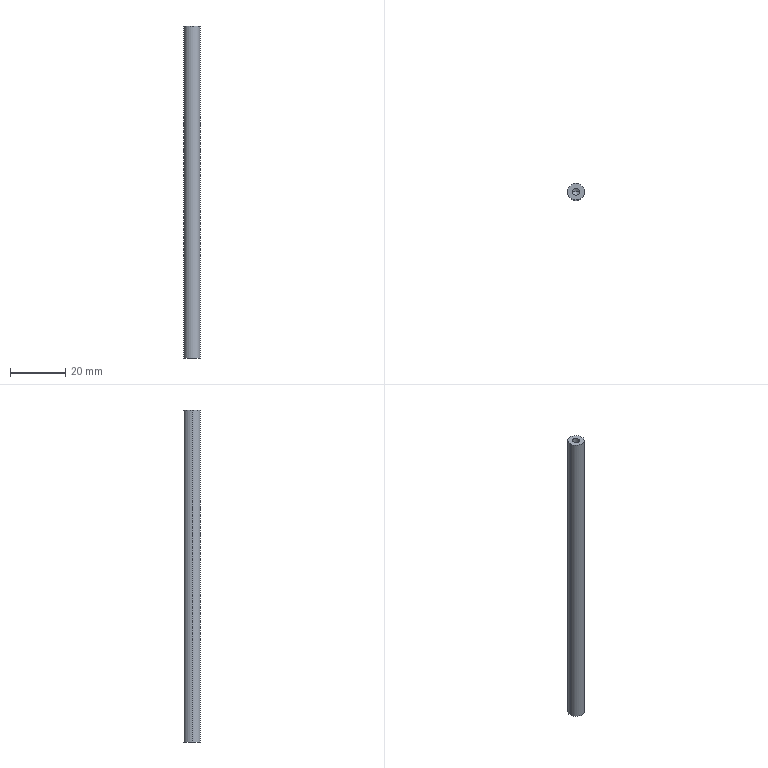Part | SolidWorks | features HoleWzd 2, Extrusion 1 | 1 solid | 12 faces | box 6 x 6 x 120 mm | volume 3307 mm3 | cylinder 6 | cone 4 | plane 2 | commonest cylinder face diameters 2.5 x4 6 x2
STEP:
#1=CARTESIAN_POINT('',(1.25,0.,8.5));
#2=VERTEX_POINT('',#1);
#3=CARTESIAN_POINT('',(-1.25,0.,8.5));
#4=VERTEX_POINT('',#3);
#5=CARTESIAN_POINT('',(0.,0.,8.5));
#6=DIRECTION('',(0.,0.,-1.));
#7=DIRECTION('',(-1.,0.,0.));
#8=AXIS2_PLACEMENT_3D('',#5,#6,#7);
#9=CIRCLE('',#8,1.25);
#10=EDGE_CURVE('',#2,#4,#9,.T.);
#11=ORIENTED_EDGE('',*,*,#10,.F.);
#12=CARTESIAN_POINT('',(1.25,0.,0.));
#13=VERTEX_POINT('',#12);
#14=CARTESIAN_POINT('',(1.25,0.,0.));
#15=DIRECTION('',(0.,0.,-1.));
#16=VECTOR('',#15,1000.);
#17=LINE('',#14,#16);
#18=EDGE_CURVE('',#2,#13,#17,.T.);
#19=ORIENTED_EDGE('',*,*,#18,.T.);
#20=CARTESIAN_POINT('',(-1.25,0.,0.));
#21=VERTEX_POINT('',#20);
#22=CARTESIAN_POINT('',(0.,0.,0.));
#23=DIRECTION('',(0.,0.,-1.));
#24=DIRECTION('',(-1.,0.,0.));
#25=AXIS2_PLACEMENT_3D('',#22,#23,#24);
#26=CIRCLE('',#25,1.25);
#27=EDGE_CURVE('',#13,#21,#26,.T.);
#28=ORIENTED_EDGE('',*,*,#27,.T.);
#29=CARTESIAN_POINT('',(-1.25,0.,0.));
#30=DIRECTION('',(0.,0.,-1.));
#31=VECTOR('',#30,1000.);
#32=LINE('',#29,#31);
#33=EDGE_CURVE('',#4,#21,#32,.T.);
#34=ORIENTED_EDGE('',*,*,#33,.F.);
#35=EDGE_LOOP('',(#11,#19,#28,#34));
#36=FACE_OUTER_BOUND('',#35,.T.);
#37=CARTESIAN_POINT('',(0.,0.,0.));
#38=DIRECTION('',(0.,0.,-1.));
#39=DIRECTION('',(-1.,0.,0.));
#40=AXIS2_PLACEMENT_3D('',#37,#38,#39);
#41=CYLINDRICAL_SURFACE('',#40,1.25);
#42=ADVANCED_FACE('',(#36),#41,.F.);
#43=CARTESIAN_POINT('',(0.,0.,9.251));
#44=VERTEX_POINT('',#43);
#45=CARTESIAN_POINT('',(-1.25,0.,8.5));
#46=DIRECTION('',(-0.8572,0.,-0.515));
#47=VECTOR('',#46,1000.);
#48=LINE('',#45,#47);
#49=EDGE_CURVE('',#44,#4,#48,.T.);
#50=ORIENTED_EDGE('',*,*,#49,.F.);
#51=CARTESIAN_POINT('',(1.25,0.,8.5));
#52=DIRECTION('',(0.8572,0.,-0.515));
#53=VECTOR('',#52,1000.);
#54=LINE('',#51,#53);
#55=EDGE_CURVE('',#44,#2,#54,.T.);
#56=ORIENTED_EDGE('',*,*,#55,.T.);
#57=ORIENTED_EDGE('',*,*,#10,.T.);
#58=EDGE_LOOP('',(#50,#56,#57));
#59=FACE_OUTER_BOUND('',#58,.T.);
#60=CARTESIAN_POINT('',(0.,0.,8.5));
#61=DIRECTION('',(0.,0.,-1.));
#62=DIRECTION('',(-1.,0.,0.));
#63=AXIS2_PLACEMENT_3D('',#60,#61,#62);
#64=CONICAL_SURFACE('',#63,1.25,1.03);
#65=ADVANCED_FACE('',(#59),#64,.F.);
#66=CARTESIAN_POINT('',(-1.25,0.,111.5));
#67=VERTEX_POINT('',#66);
#68=CARTESIAN_POINT('',(1.25,0.,111.5));
#69=VERTEX_POINT('',#68);
#70=CARTESIAN_POINT('',(0.,0.,111.5));
#71=DIRECTION('',(0.,0.,1.));
#72=DIRECTION('',(1.,0.,0.));
#73=AXIS2_PLACEMENT_3D('',#70,#71,#72);
#74=CIRCLE('',#73,1.25);
#75=EDGE_CURVE('',#67,#69,#74,.T.);
#76=ORIENTED_EDGE('',*,*,#75,.F.);
#77=CARTESIAN_POINT('',(-1.25,0.,120.));
#78=VERTEX_POINT('',#77);
#79=CARTESIAN_POINT('',(-1.25,0.,120.));
#80=DIRECTION('',(0.,0.,1.));
#81=VECTOR('',#80,1000.);
#82=LINE('',#79,#81);
#83=EDGE_CURVE('',#67,#78,#82,.T.);
#84=ORIENTED_EDGE('',*,*,#83,.T.);
#85=CARTESIAN_POINT('',(1.25,0.,120.));
#86=VERTEX_POINT('',#85);
#87=CARTESIAN_POINT('',(0.,0.,120.));
#88=DIRECTION('',(0.,0.,1.));
#89=DIRECTION('',(1.,0.,0.));
#90=AXIS2_PLACEMENT_3D('',#87,#88,#89);
#91=CIRCLE('',#90,1.25);
#92=EDGE_CURVE('',#78,#86,#91,.T.);
#93=ORIENTED_EDGE('',*,*,#92,.T.);
#94=CARTESIAN_POINT('',(1.25,0.,120.));
#95=DIRECTION('',(0.,0.,1.));
#96=VECTOR('',#95,1000.);
#97=LINE('',#94,#96);
#98=EDGE_CURVE('',#69,#86,#97,.T.);
#99=ORIENTED_EDGE('',*,*,#98,.F.);
#100=EDGE_LOOP('',(#76,#84,#93,#99));
#101=FACE_OUTER_BOUND('',#100,.T.);
#102=CARTESIAN_POINT('',(0.,0.,120.));
#103=DIRECTION('',(0.,0.,1.));
#104=DIRECTION('',(1.,0.,0.));
#105=AXIS2_PLACEMENT_3D('',#102,#103,#104);
#106=CYLINDRICAL_SURFACE('',#105,1.25);
#107=ADVANCED_FACE('',(#101),#106,.F.);
#108=CARTESIAN_POINT('',(0.,0.,110.749));
#109=VERTEX_POINT('',#108);
#110=CARTESIAN_POINT('',(1.25,0.,111.5));
#111=DIRECTION('',(0.8572,0.,0.515));
#112=VECTOR('',#111,1000.);
#113=LINE('',#110,#112);
#114=EDGE_CURVE('',#109,#69,#113,.T.);
#115=ORIENTED_EDGE('',*,*,#114,.F.);
#116=CARTESIAN_POINT('',(-1.25,0.,111.5));
#117=DIRECTION('',(-0.8572,0.,0.515));
#118=VECTOR('',#117,1000.);
#119=LINE('',#116,#118);
#120=EDGE_CURVE('',#109,#67,#119,.T.);
#121=ORIENTED_EDGE('',*,*,#120,.T.);
#122=ORIENTED_EDGE('',*,*,#75,.T.);
#123=EDGE_LOOP('',(#115,#121,#122));
#124=FACE_OUTER_BOUND('',#123,.T.);
#125=CARTESIAN_POINT('',(0.,0.,111.5));
#126=DIRECTION('',(0.,0.,1.));
#127=DIRECTION('',(1.,0.,0.));
#128=AXIS2_PLACEMENT_3D('',#125,#126,#127);
#129=CONICAL_SURFACE('',#128,1.25,1.03);
#130=ADVANCED_FACE('',(#124),#129,.F.);
#131=CARTESIAN_POINT('',(3.,0.,120.));
#132=VERTEX_POINT('',#131);
#133=CARTESIAN_POINT('',(-3.,0.,120.));
#134=VERTEX_POINT('',#133);
#135=CARTESIAN_POINT('',(0.,0.,120.));
#136=DIRECTION('',(0.,0.,1.));
#137=DIRECTION('',(1.,0.,0.));
#138=AXIS2_PLACEMENT_3D('',#135,#136,#137);
#139=CIRCLE('',#138,3.);
#140=EDGE_CURVE('',#132,#134,#139,.T.);
#141=ORIENTED_EDGE('',*,*,#140,.F.);
#142=CARTESIAN_POINT('',(3.,0.,0.));
#143=VERTEX_POINT('',#142);
#144=CARTESIAN_POINT('',(3.,0.,120.));
#145=DIRECTION('',(0.,0.,-1.));
#146=VECTOR('',#145,1000.);
#147=LINE('',#144,#146);
#148=EDGE_CURVE('',#132,#143,#147,.T.);
#149=ORIENTED_EDGE('',*,*,#148,.T.);
#150=CARTESIAN_POINT('',(-3.,0.,0.));
#151=VERTEX_POINT('',#150);
#152=CARTESIAN_POINT('',(0.,0.,0.));
#153=DIRECTION('',(0.,0.,1.));
#154=DIRECTION('',(1.,0.,0.));
#155=AXIS2_PLACEMENT_3D('',#152,#153,#154);
#156=CIRCLE('',#155,3.);
#157=EDGE_CURVE('',#143,#151,#156,.T.);
#158=ORIENTED_EDGE('',*,*,#157,.T.);
#159=CARTESIAN_POINT('',(-3.,0.,120.));
#160=DIRECTION('',(0.,0.,-1.));
#161=VECTOR('',#160,1000.);
#162=LINE('',#159,#161);
#163=EDGE_CURVE('',#134,#151,#162,.T.);
#164=ORIENTED_EDGE('',*,*,#163,.F.);
#165=EDGE_LOOP('',(#141,#149,#158,#164));
#166=FACE_OUTER_BOUND('',#165,.T.);
#167=CARTESIAN_POINT('',(0.,0.,120.));
#168=DIRECTION('',(0.,0.,-1.));
#169=DIRECTION('',(-1.,0.,0.));
#170=AXIS2_PLACEMENT_3D('',#167,#168,#169);
#171=CYLINDRICAL_SURFACE('',#170,3.);
#172=ADVANCED_FACE('',(#166),#171,.T.);
#173=ORIENTED_EDGE('',*,*,#148,.F.);
#174=CARTESIAN_POINT('',(0.,0.,120.));
#175=DIRECTION('',(0.,0.,1.));
#176=DIRECTION('',(1.,0.,0.));
#177=AXIS2_PLACEMENT_3D('',#174,#175,#176);
#178=CIRCLE('',#177,3.);
#179=EDGE_CURVE('',#134,#132,#178,.T.);
#180=ORIENTED_EDGE('',*,*,#179,.F.);
#181=ORIENTED_EDGE('',*,*,#163,.T.);
#182=CARTESIAN_POINT('',(0.,0.,0.));
#183=DIRECTION('',(0.,0.,1.));
#184=DIRECTION('',(1.,0.,0.));
#185=AXIS2_PLACEMENT_3D('',#182,#183,#184);
#186=CIRCLE('',#185,3.);
#187=EDGE_CURVE('',#151,#143,#186,.T.);
#188=ORIENTED_EDGE('',*,*,#187,.T.);
#189=EDGE_LOOP('',(#173,#180,#181,#188));
#190=FACE_OUTER_BOUND('',#189,.T.);
#191=CARTESIAN_POINT('',(0.,0.,120.));
#192=DIRECTION('',(0.,0.,-1.));
#193=DIRECTION('',(-1.,0.,0.));
#194=AXIS2_PLACEMENT_3D('',#191,#192,#193);
#195=CYLINDRICAL_SURFACE('',#194,3.);
#196=ADVANCED_FACE('',(#190),#195,.T.);
#197=CARTESIAN_POINT('',(0.,0.,120.));
#198=DIRECTION('',(0.,0.,1.));
#199=DIRECTION('',(1.,0.,0.));
#200=AXIS2_PLACEMENT_3D('',#197,#198,#199);
#201=CIRCLE('',#200,1.25);
#202=EDGE_CURVE('',#86,#78,#201,.T.);
#203=ORIENTED_EDGE('',*,*,#202,.F.);
#204=ORIENTED_EDGE('',*,*,#92,.F.);
#205=EDGE_LOOP('',(#203,#204));
#206=FACE_BOUND('',#205,.T.);
#207=ORIENTED_EDGE('',*,*,#179,.T.);
#208=ORIENTED_EDGE('',*,*,#140,.T.);
#209=EDGE_LOOP('',(#207,#208));
#210=FACE_OUTER_BOUND('',#209,.T.);
#211=CARTESIAN_POINT('',(0.,0.,120.));
#212=DIRECTION('',(0.,0.,1.));
#213=DIRECTION('',(1.,0.,0.));
#214=AXIS2_PLACEMENT_3D('',#211,#212,#213);
#215=PLANE('',#214);
#216=ADVANCED_FACE('',(#206,#210),#215,.T.);
#217=CARTESIAN_POINT('',(0.,0.,0.));
#218=DIRECTION('',(0.,0.,-1.));
#219=DIRECTION('',(-1.,0.,0.));
#220=AXIS2_PLACEMENT_3D('',#217,#218,#219);
#221=CIRCLE('',#220,1.25);
#222=EDGE_CURVE('',#21,#13,#221,.T.);
#223=ORIENTED_EDGE('',*,*,#222,.F.);
#224=ORIENTED_EDGE('',*,*,#27,.F.);
#225=EDGE_LOOP('',(#223,#224));
#226=FACE_BOUND('',#225,.T.);
#227=ORIENTED_EDGE('',*,*,#187,.F.);
#228=ORIENTED_EDGE('',*,*,#157,.F.);
#229=EDGE_LOOP('',(#227,#228));
#230=FACE_OUTER_BOUND('',#229,.T.);
#231=CARTESIAN_POINT('',(0.,0.,0.));
#232=DIRECTION('',(0.,0.,1.));
#233=DIRECTION('',(1.,0.,0.));
#234=AXIS2_PLACEMENT_3D('',#231,#232,#233);
#235=PLANE('',#234);
#236=ADVANCED_FACE('',(#226,#230),#235,.F.);
#237=ORIENTED_EDGE('',*,*,#120,.F.);
#238=ORIENTED_EDGE('',*,*,#114,.T.);
#239=CARTESIAN_POINT('',(0.,0.,111.5));
#240=DIRECTION('',(0.,0.,1.));
#241=DIRECTION('',(1.,0.,0.));
#242=AXIS2_PLACEMENT_3D('',#239,#240,#241);
#243=CIRCLE('',#242,1.25);
#244=EDGE_CURVE('',#69,#67,#243,.T.);
#245=ORIENTED_EDGE('',*,*,#244,.T.);
#246=EDGE_LOOP('',(#237,#238,#245));
#247=FACE_OUTER_BOUND('',#246,.T.);
#248=CARTESIAN_POINT('',(0.,0.,111.5));
#249=DIRECTION('',(0.,0.,1.));
#250=DIRECTION('',(1.,0.,0.));
#251=AXIS2_PLACEMENT_3D('',#248,#249,#250);
#252=CONICAL_SURFACE('',#251,1.25,1.03);
#253=ADVANCED_FACE('',(#247),#252,.F.);
#254=ORIENTED_EDGE('',*,*,#83,.F.);
#255=ORIENTED_EDGE('',*,*,#244,.F.);
#256=ORIENTED_EDGE('',*,*,#98,.T.);
#257=ORIENTED_EDGE('',*,*,#202,.T.);
#258=EDGE_LOOP('',(#254,#255,#256,#257));
#259=FACE_OUTER_BOUND('',#258,.T.);
#260=CARTESIAN_POINT('',(0.,0.,120.));
#261=DIRECTION('',(0.,0.,1.));
#262=DIRECTION('',(1.,0.,0.));
#263=AXIS2_PLACEMENT_3D('',#260,#261,#262);
#264=CYLINDRICAL_SURFACE('',#263,1.25);
#265=ADVANCED_FACE('',(#259),#264,.F.);
#266=ORIENTED_EDGE('',*,*,#55,.F.);
#267=ORIENTED_EDGE('',*,*,#49,.T.);
#268=CARTESIAN_POINT('',(0.,0.,8.5));
#269=DIRECTION('',(0.,0.,-1.));
#270=DIRECTION('',(-1.,0.,0.));
#271=AXIS2_PLACEMENT_3D('',#268,#269,#270);
#272=CIRCLE('',#271,1.25);
#273=EDGE_CURVE('',#4,#2,#272,.T.);
#274=ORIENTED_EDGE('',*,*,#273,.T.);
#275=EDGE_LOOP('',(#266,#267,#274));
#276=FACE_OUTER_BOUND('',#275,.T.);
#277=CARTESIAN_POINT('',(0.,0.,8.5));
#278=DIRECTION('',(0.,0.,-1.));
#279=DIRECTION('',(-1.,0.,0.));
#280=AXIS2_PLACEMENT_3D('',#277,#278,#279);
#281=CONICAL_SURFACE('',#280,1.25,1.03);
#282=ADVANCED_FACE('',(#276),#281,.F.);
#283=ORIENTED_EDGE('',*,*,#18,.F.);
#284=ORIENTED_EDGE('',*,*,#273,.F.);
#285=ORIENTED_EDGE('',*,*,#33,.T.);
#286=ORIENTED_EDGE('',*,*,#222,.T.);
#287=EDGE_LOOP('',(#283,#284,#285,#286));
#288=FACE_OUTER_BOUND('',#287,.T.);
#289=CARTESIAN_POINT('',(0.,0.,0.));
#290=DIRECTION('',(0.,0.,-1.));
#291=DIRECTION('',(-1.,0.,0.));
#292=AXIS2_PLACEMENT_3D('',#289,#290,#291);
#293=CYLINDRICAL_SURFACE('',#292,1.25);
#294=ADVANCED_FACE('',(#288),#293,.F.);
#295=CLOSED_SHELL('',(#42,#65,#107,#130,#172,#196,#216,#236,#253,#265,#282,#294));
#296=MANIFOLD_SOLID_BREP('',#295);
#297=CARTESIAN_POINT('',(0.,0.,0.));
#298=DIRECTION('',(0.,0.,1.));
#299=DIRECTION('',(1.,0.,0.));
#300=AXIS2_PLACEMENT_3D('',#297,#298,#299);
#301=(LENGTH_UNIT()NAMED_UNIT(*)SI_UNIT(.MILLI.,.METRE.));
#302=UNCERTAINTY_MEASURE_WITH_UNIT(LENGTH_MEASURE(0.00001),#301,'','');
#303=(NAMED_UNIT(*)PLANE_ANGLE_UNIT()SI_UNIT($,.RADIAN.));
#304=(NAMED_UNIT(*)SI_UNIT($,.STERADIAN.)SOLID_ANGLE_UNIT());
#305=(GEOMETRIC_REPRESENTATION_CONTEXT(3)GLOBAL_UNCERTAINTY_ASSIGNED_CONTEXT((#302))GLOBAL_UNIT_ASSIGNED_CONTEXT((#301,#303,#304))REPRESENTATION_CONTEXT('',''));
#306=ADVANCED_BREP_SHAPE_REPRESENTATION('',(#296,#300),#305);